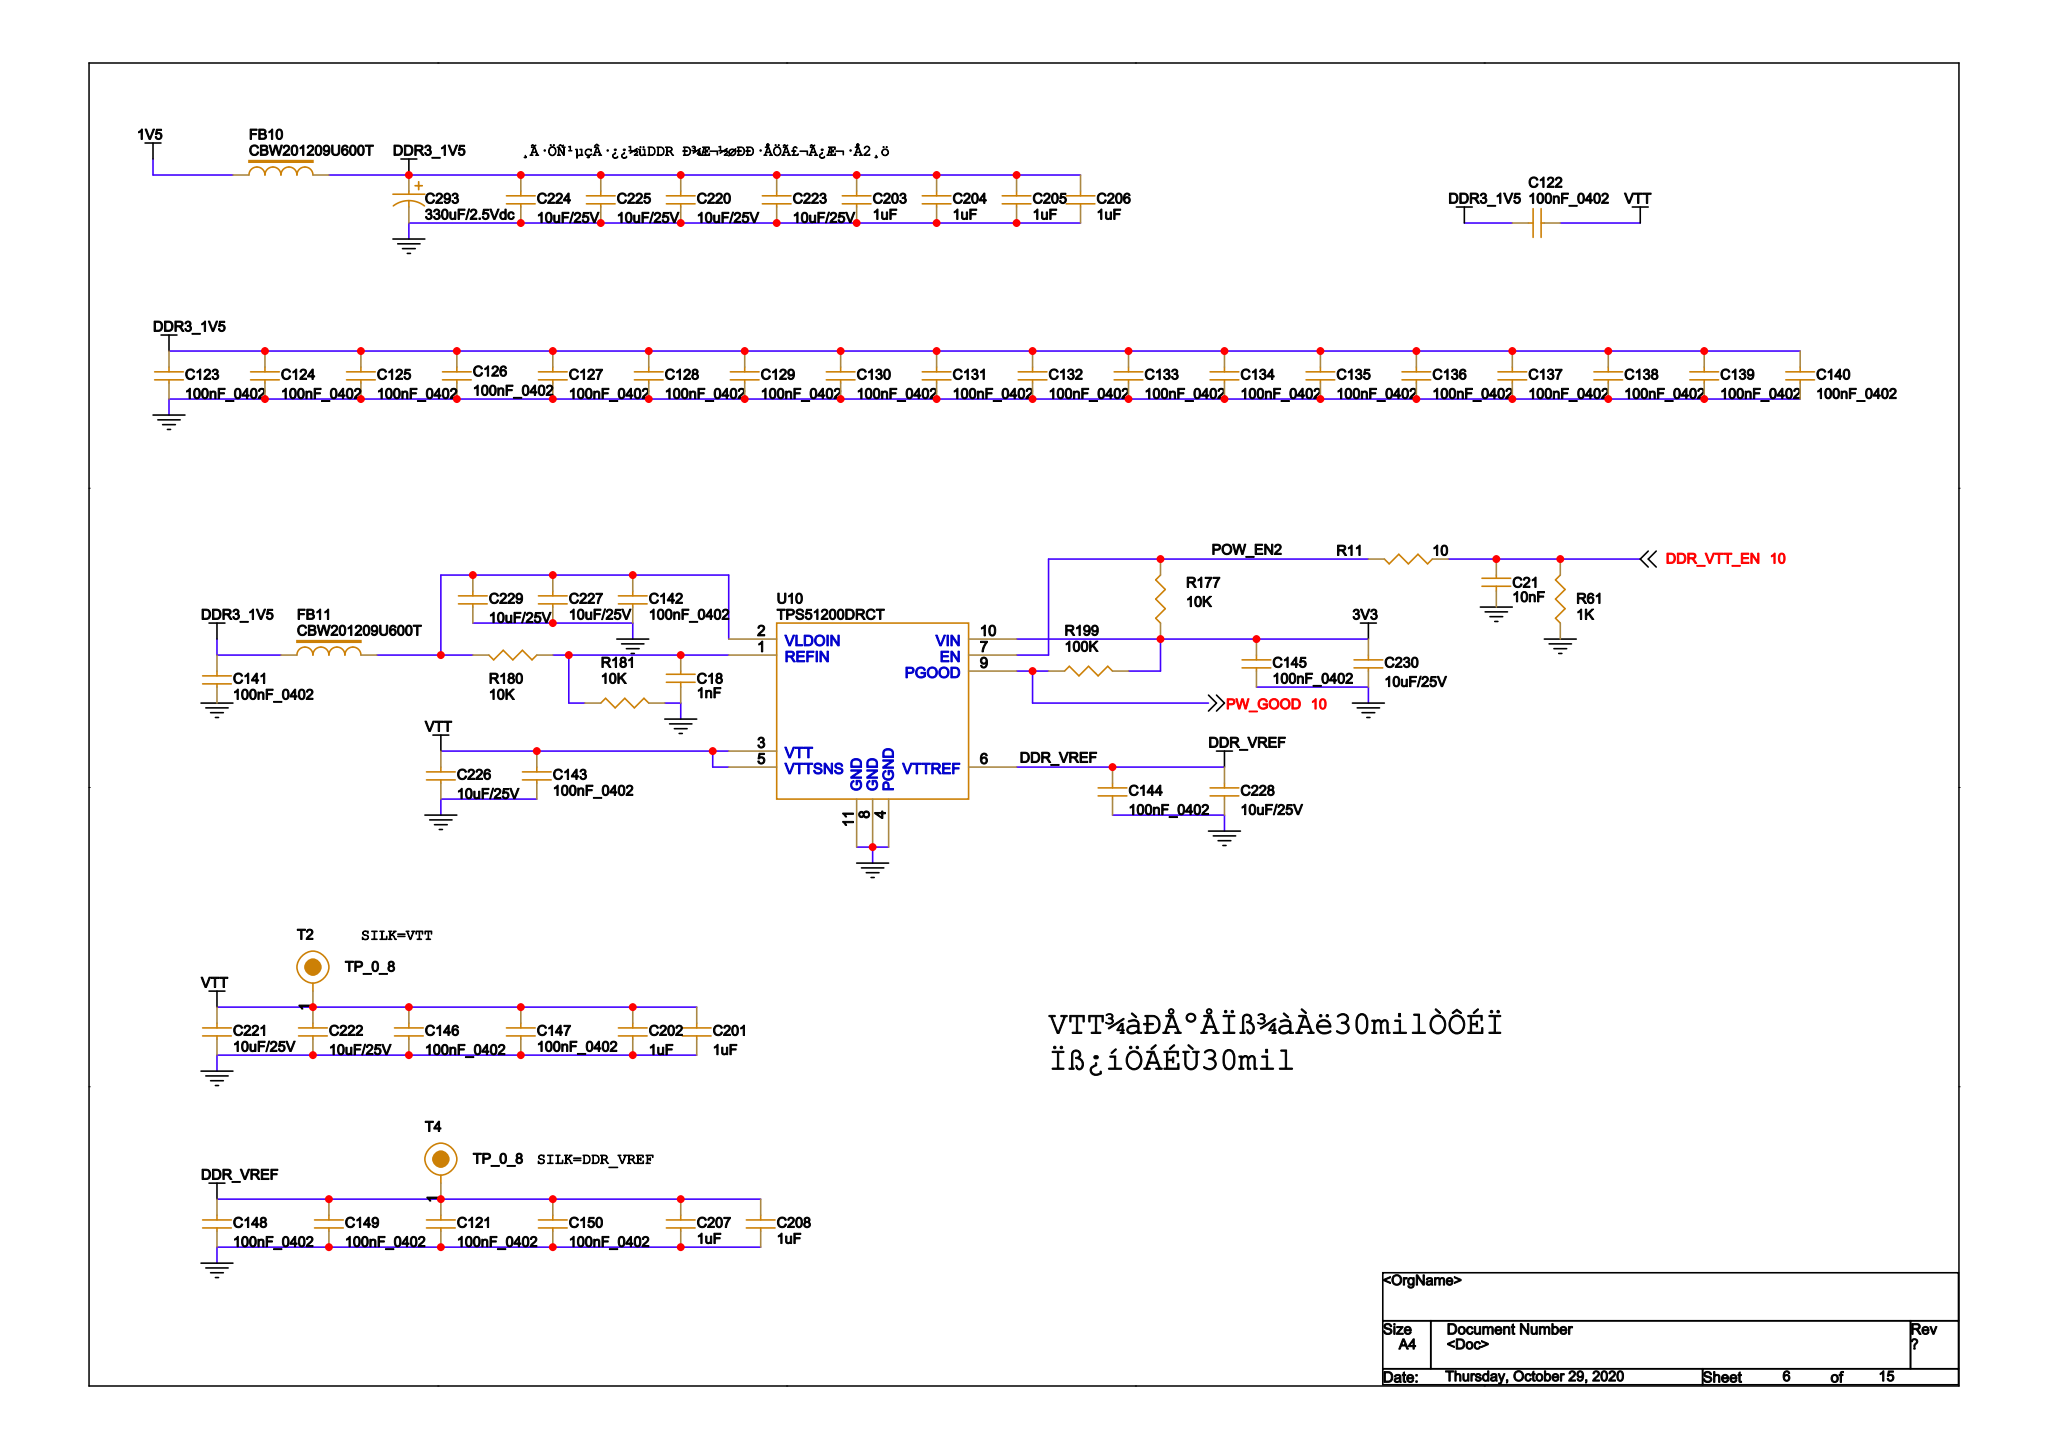Circuit board | Cadence Allegro | 406 parts | 392 nets | one sheet of the schematic
Parts on this sheet (reference | value | footprint):
C18 | 1nF | C_0603
C21 | 10nF | C_0603
C121 | 100nF_0402 | C_0402_BGA
C122 | 100nF_0402 | C_0402_BGA
C123 | 100nF_0402 | C_0402_BGA
C124 | 100nF_0402 | C_0402_BGA
C125 | 100nF_0402 | C_0402_BGA
C126 | 100nF_0402 | C_0402_BGA
C127 | 100nF_0402 | C_0402_BGA
C128 | 100nF_0402 | C_0402_BGA
C129 | 100nF_0402 | C_0402_BGA
C130 | 100nF_0402 | C_0402_BGA
C131 | 100nF_0402 | C_0402_BGA
C132 | 100nF_0402 | C_0402_BGA
C133 | 100nF_0402 | C_0402_BGA
C134 | 100nF_0402 | C_0402_BGA
C135 | 100nF_0402 | C_0402_BGA
C136 | 100nF_0402 | C_0402_BGA
C137 | 100nF_0402 | C_0402_BGA
C138 | 100nF_0402 | C_0402_BGA
C139 | 100nF_0402 | C_0402_BGA
C140 | 100nF_0402 | C_0402_BGA
C141 | 100nF_0402 | C_0402_BGA
C142 | 100nF_0402 | C_0402_BGA
C143 | 100nF_0402 | C_0402_BGA
C144 | 100nF_0402 | C_0402_BGA
C145 | 100nF_0402 | C_0402_BGA
C146 | 100nF_0402 | C_0402_BGA
C147 | 100nF_0402 | C_0402_BGA
C148 | 100nF_0402 | C_0402_BGA
C149 | 100nF_0402 | C_0402_BGA
C150 | 100nF_0402 | C_0402_BGA
C201 | 1uF | C_0603
C202 | 1uF | C_0603
C203 | 1uF | C_0603
C204 | 1uF | C_0603
C205 | 1uF | C_0603
C206 | 1uF | C_0603
C207 | 1uF | C_0603
C208 | 1uF | C_0603
C220 | 10uF/25V | C_0805_106
C221 | 10uF/25V | C_0805_106
C222 | 10uF/25V | C_0805_106
C223 | 10uF/25V | C_0805_106
C224 | 10uF/25V | C_0805_106
C225 | 10uF/25V | C_0805_106
C226 | 10uF/25V | C_0805_106
C227 | 10uF/25V | C_0805_106
C228 | 10uF/25V | C_0805_106
C229 | 10uF/25V | C_0805_106
C230 | 10uF/25V | C_0805_106
C293 | 330uF/2.5Vdc | C_7343
FB10 | CBW201209U600T | L_0805
FB11 | CBW201209U600T | L_0805
R11 | 10 | R_0603
R61 | 1K | R_0603
R177 | 10K | R_0603
R180 | 10K | R_0603
R181 | 10K | R_0603
R199 | 100K | R_0603
U10 | TPS51200DRCT | U_VSON10
Nets of these parts (net: part-pin ...):
GND: C18-2 C21-2 C121-1 C123-1 C124-1 C125-1 C126-1 C127-1 C128-1 C129-1 C130-1 C131-1 C132-1 C133-1 C134-1 C135-1 C136-1 C137-1 C138-1 C139-1 C140-1 C141-1 C142-1 C143-1 C144-1 C145-1 C146-1 C147-1 C148-1 C149-1 C150-1 C201-1 C202-1 C203-1 C204-1 C205-1 C206-1 C207-1 C208-1 C220-1 C221-1 C222-1 C223-1 C224-1 C225-1 C226-1 C227-1 C228-1 C229-1 C230-1 C293-2 R61-1 R181-2 U10-4 U10-8 U10-11
DDR3_1V5: C122-2 C123-2 C124-2 C125-2 C126-2 C127-2 C128-2 C129-2 C130-2 C131-2 C132-2 C133-2 C134-2 C135-2 C136-2 C137-2 C138-2 C139-2 C140-2 C141-2 C203-2 C204-2 C205-2 C206-2 C220-2 C223-2 C224-2 C225-2 C293-1 FB10-2 FB11-1
VTT: C122-1 C143-2 C146-2 C147-2 C201-2 C202-2 C221-2 C222-2 C226-2 U10-3 U10-5
DDR_VREF: C121-2 C144-2 C148-2 C149-2 C150-2 C207-2 C208-2 C228-2 U10-6
N16565440: C142-2 C227-2 C229-2 FB11-2 R180-2 U10-2
3V3: C145-2 C230-2 R177-1 R199-2 U10-10
1V5: FB10-1
N18651238: C18-1 R180-1 R181-1 U10-1
DDR_VTT_EN: C21-1 R11-1 R61-2
POW_EN2: R11-2 R177-2 U10-7
PW_GOOD: R199-1 U10-9